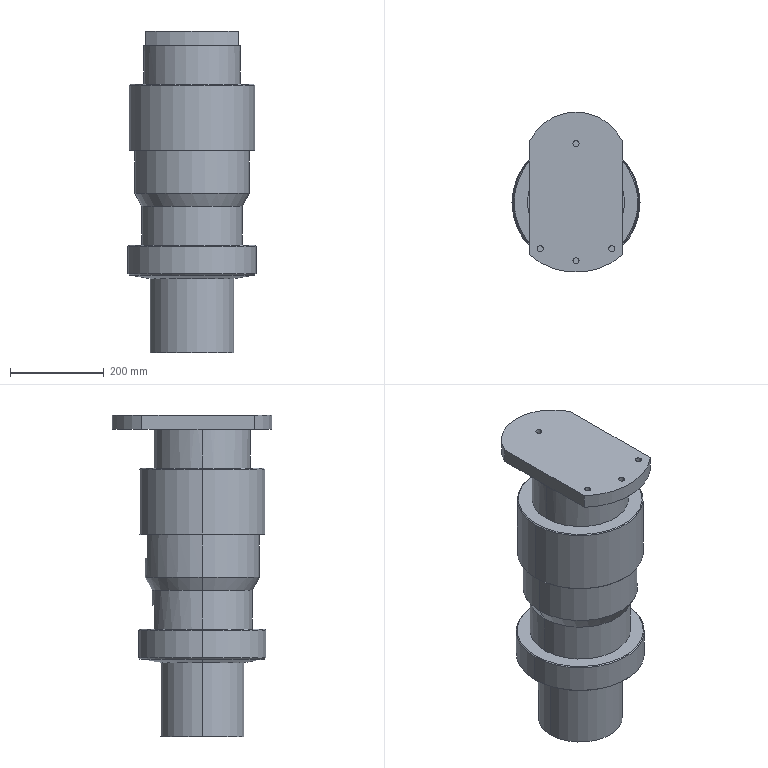Part | SolidWorks | features ICE 4, Chamfer 2, Extrusion 1, RefAxis 1, Revolution 1 | 1 solid | 72 faces | box 273 x 341.706 x 685 mm | volume 8218531 mm3 | cylinder 36 | plane 24 | cone 12 | commonest cylinder face diameters 13 x8 244 x4 155 x2 179 x2 180 x2 186 x2